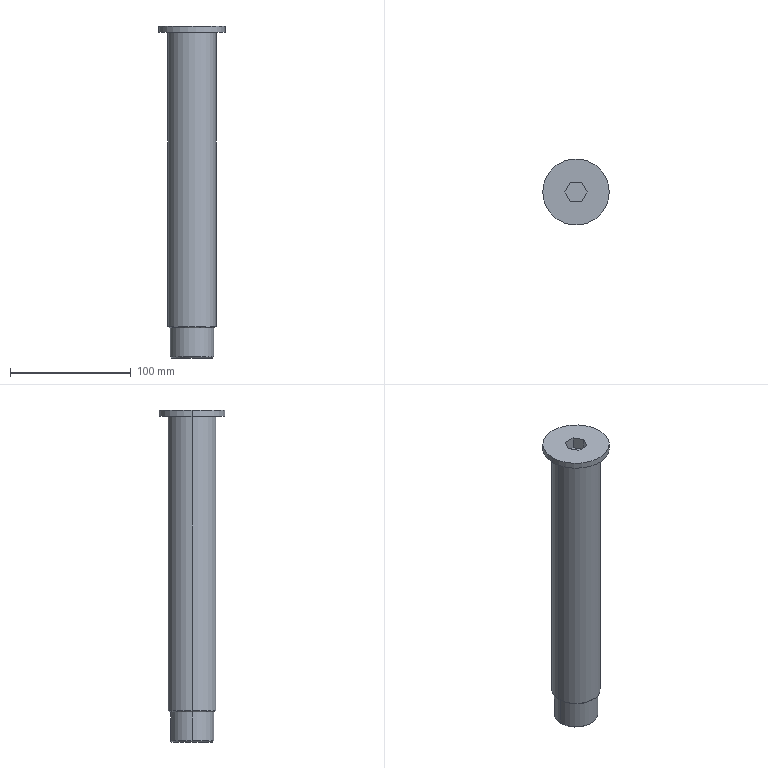Part | SolidWorks | features ICE 4, Chamfer 2, Fillet 2, Extrusion 1 | 1 solid | 32 faces | box 55 x 55 x 275 mm | volume 342139 mm3 | plane 14 | cylinder 11 | cone 5 | torus 2 | commonest cylinder face diameters 1 x4 36 x3 40 x2 55 x2
STEP:
#1=CARTESIAN_POINT('',(-20.5,0.,270.));
#2=VERTEX_POINT('',#1);
#3=CARTESIAN_POINT('',(20.5,0.,270.));
#4=VERTEX_POINT('',#3);
#5=CARTESIAN_POINT('',(0.,0.,270.));
#6=DIRECTION('',(0.,0.,1.));
#7=DIRECTION('',(1.,0.,0.));
#8=AXIS2_PLACEMENT_3D('',#5,#6,#7);
#9=CIRCLE('',#8,20.5);
#10=EDGE_CURVE('',#2,#4,#9,.T.);
#11=ORIENTED_EDGE('',*,*,#10,.F.);
#12=CARTESIAN_POINT('',(-20.,0.,269.5));
#13=VERTEX_POINT('',#12);
#14=CARTESIAN_POINT('',(-20.5,0.,269.5));
#15=DIRECTION('',(0.,1.,0.));
#16=DIRECTION('',(-1.,0.,0.));
#17=AXIS2_PLACEMENT_3D('',#14,#15,#16);
#18=CIRCLE('',#17,0.5);
#19=EDGE_CURVE('',#2,#13,#18,.T.);
#20=ORIENTED_EDGE('',*,*,#19,.T.);
#21=CARTESIAN_POINT('',(20.,0.,269.5));
#22=VERTEX_POINT('',#21);
#23=CARTESIAN_POINT('',(0.,0.,269.5));
#24=DIRECTION('',(0.,0.,-1.));
#25=DIRECTION('',(1.,0.,0.));
#26=AXIS2_PLACEMENT_3D('',#23,#24,#25);
#27=CIRCLE('',#26,20.);
#28=EDGE_CURVE('',#22,#13,#27,.T.);
#29=ORIENTED_EDGE('',*,*,#28,.F.);
#30=CARTESIAN_POINT('',(20.5,0.,269.5));
#31=DIRECTION('',(0.,-1.,0.));
#32=DIRECTION('',(0.,0.,-1.));
#33=AXIS2_PLACEMENT_3D('',#30,#31,#32);
#34=CIRCLE('',#33,0.5);
#35=EDGE_CURVE('',#4,#22,#34,.T.);
#36=ORIENTED_EDGE('',*,*,#35,.F.);
#37=EDGE_LOOP('',(#11,#20,#29,#36));
#38=FACE_OUTER_BOUND('',#37,.T.);
#39=CARTESIAN_POINT('',(0.,0.,269.5));
#40=DIRECTION('',(0.,0.,1.));
#41=DIRECTION('',(1.,0.,0.));
#42=AXIS2_PLACEMENT_3D('',#39,#40,#41);
#43=TOROIDAL_SURFACE('',#42,20.5,0.5);
#44=ADVANCED_FACE('',(#38),#43,.F.);
#45=CARTESIAN_POINT('',(-17.,0.,0.));
#46=VERTEX_POINT('',#45);
#47=CARTESIAN_POINT('',(-3.,16.733,0.));
#48=VERTEX_POINT('',#47);
#49=CARTESIAN_POINT('',(0.,0.,0.));
#50=DIRECTION('',(0.,0.,-1.));
#51=DIRECTION('',(1.,0.,0.));
#52=AXIS2_PLACEMENT_3D('',#49,#50,#51);
#53=CIRCLE('',#52,17.);
#54=EDGE_CURVE('',#46,#48,#53,.T.);
#55=ORIENTED_EDGE('',*,*,#54,.F.);
#56=CARTESIAN_POINT('',(-18.,0.,1.));
#57=VERTEX_POINT('',#56);
#58=CARTESIAN_POINT('',(-17.,0.,0.));
#59=DIRECTION('',(-0.7071,0.,0.7071));
#60=VECTOR('',#59,1000.);
#61=LINE('',#58,#60);
#62=EDGE_CURVE('',#46,#57,#61,.T.);
#63=ORIENTED_EDGE('',*,*,#62,.T.);
#64=CARTESIAN_POINT('',(-3.6,17.636,1.));
#65=VERTEX_POINT('',#64);
#66=CARTESIAN_POINT('',(0.,0.,1.));
#67=DIRECTION('',(0.,0.,1.));
#68=DIRECTION('',(1.,0.,0.));
#69=AXIS2_PLACEMENT_3D('',#66,#67,#68);
#70=CIRCLE('',#69,18.);
#71=EDGE_CURVE('',#65,#57,#70,.T.);
#72=ORIENTED_EDGE('',*,*,#71,.F.);
#73=CARTESIAN_POINT('',(-3.,17.146,0.4069));
#74=VERTEX_POINT('',#73);
#75=CARTESIAN_POINT('',(-3.6,17.636,1.));
#76=CARTESIAN_POINT('',(-3.509,17.655,1.));
#77=CARTESIAN_POINT('',(-3.418,17.647,0.9743));
#78=CARTESIAN_POINT('',(-3.262,17.594,0.8932));
#79=CARTESIAN_POINT('',(-3.198,17.551,0.8399));
#80=CARTESIAN_POINT('',(-3.098,17.452,0.7251));
#81=CARTESIAN_POINT('',(-3.061,17.395,0.6623));
#82=CARTESIAN_POINT('',(-3.013,17.275,0.5357));
#83=CARTESIAN_POINT('',(-3.,17.212,0.4712));
#84=CARTESIAN_POINT('',(-3.,17.146,0.4069));
#85=B_SPLINE_CURVE_WITH_KNOTS('',3,(#75,#76,#77,#78,#79,#80,#81,#82,#83,#84),.UNSPECIFIED.,.F.,.F.,(4,2,2,2,4),(0.,0.0002726,0.0005452,0.0008178,0.00109),.UNSPECIFIED.);
#86=EDGE_CURVE('',#65,#74,#85,.T.);
#87=ORIENTED_EDGE('',*,*,#86,.T.);
#88=CARTESIAN_POINT('',(-3.,16.733,0.));
#89=CARTESIAN_POINT('',(-3.,16.871,0.1356));
#90=CARTESIAN_POINT('',(-3.,17.009,0.2712));
#91=CARTESIAN_POINT('',(-3.,17.146,0.4069));
#92=B_SPLINE_CURVE_WITH_KNOTS('',3,(#88,#89,#90,#91),.UNSPECIFIED.,.F.,.F.,(4,4),(0.007295,0.007875),.UNSPECIFIED.);
#93=EDGE_CURVE('',#48,#74,#92,.T.);
#94=ORIENTED_EDGE('',*,*,#93,.F.);
#95=EDGE_LOOP('',(#55,#63,#72,#87,#94));
#96=FACE_OUTER_BOUND('',#95,.T.);
#97=CARTESIAN_POINT('',(0.,0.,0.));
#98=DIRECTION('',(0.,0.,1.));
#99=DIRECTION('',(1.,0.,0.));
#100=AXIS2_PLACEMENT_3D('',#97,#98,#99);
#101=CONICAL_SURFACE('',#100,17.,0.7854);
#102=ADVANCED_FACE('',(#96),#101,.T.);
#103=ORIENTED_EDGE('',*,*,#62,.F.);
#104=CARTESIAN_POINT('',(17.,0.,0.));
#105=VERTEX_POINT('',#104);
#106=CARTESIAN_POINT('',(0.,0.,0.));
#107=DIRECTION('',(0.,0.,-1.));
#108=DIRECTION('',(1.,0.,0.));
#109=AXIS2_PLACEMENT_3D('',#106,#107,#108);
#110=CIRCLE('',#109,17.);
#111=EDGE_CURVE('',#105,#46,#110,.T.);
#112=ORIENTED_EDGE('',*,*,#111,.F.);
#113=CARTESIAN_POINT('',(18.,0.,1.));
#114=VERTEX_POINT('',#113);
#115=CARTESIAN_POINT('',(17.,0.,0.));
#116=DIRECTION('',(0.7071,0.,0.7071));
#117=VECTOR('',#116,1000.);
#118=LINE('',#115,#117);
#119=EDGE_CURVE('',#105,#114,#118,.T.);
#120=ORIENTED_EDGE('',*,*,#119,.T.);
#121=CARTESIAN_POINT('',(0.,0.,1.));
#122=DIRECTION('',(0.,0.,1.));
#123=DIRECTION('',(1.,0.,0.));
#124=AXIS2_PLACEMENT_3D('',#121,#122,#123);
#125=CIRCLE('',#124,18.);
#126=EDGE_CURVE('',#57,#114,#125,.T.);
#127=ORIENTED_EDGE('',*,*,#126,.F.);
#128=EDGE_LOOP('',(#103,#112,#120,#127));
#129=FACE_OUTER_BOUND('',#128,.T.);
#130=CARTESIAN_POINT('',(0.,0.,0.));
#131=DIRECTION('',(0.,0.,1.));
#132=DIRECTION('',(1.,0.,0.));
#133=AXIS2_PLACEMENT_3D('',#130,#131,#132);
#134=CONICAL_SURFACE('',#133,17.,0.7854);
#135=ADVANCED_FACE('',(#129),#134,.T.);
#136=CARTESIAN_POINT('',(-19.,0.,25.));
#137=VERTEX_POINT('',#136);
#138=CARTESIAN_POINT('',(19.,0.,25.));
#139=VERTEX_POINT('',#138);
#140=CARTESIAN_POINT('',(0.,0.,25.));
#141=DIRECTION('',(0.,0.,-1.));
#142=DIRECTION('',(-1.,0.,0.));
#143=AXIS2_PLACEMENT_3D('',#140,#141,#142);
#144=CIRCLE('',#143,19.);
#145=EDGE_CURVE('',#137,#139,#144,.T.);
#146=ORIENTED_EDGE('',*,*,#145,.F.);
#147=CARTESIAN_POINT('',(-20.,0.,26.));
#148=VERTEX_POINT('',#147);
#149=CARTESIAN_POINT('',(-19.,0.,25.));
#150=DIRECTION('',(-0.7071,0.,0.7071));
#151=VECTOR('',#150,1000.);
#152=LINE('',#149,#151);
#153=EDGE_CURVE('',#137,#148,#152,.T.);
#154=ORIENTED_EDGE('',*,*,#153,.T.);
#155=CARTESIAN_POINT('',(20.,0.,26.));
#156=VERTEX_POINT('',#155);
#157=CARTESIAN_POINT('',(0.,0.,26.));
#158=DIRECTION('',(0.,0.,1.));
#159=DIRECTION('',(-1.,0.,0.));
#160=AXIS2_PLACEMENT_3D('',#157,#158,#159);
#161=CIRCLE('',#160,20.);
#162=EDGE_CURVE('',#156,#148,#161,.T.);
#163=ORIENTED_EDGE('',*,*,#162,.F.);
#164=CARTESIAN_POINT('',(19.,0.,25.));
#165=DIRECTION('',(0.7071,0.,0.7071));
#166=VECTOR('',#165,1000.);
#167=LINE('',#164,#166);
#168=EDGE_CURVE('',#139,#156,#167,.T.);
#169=ORIENTED_EDGE('',*,*,#168,.F.);
#170=EDGE_LOOP('',(#146,#154,#163,#169));
#171=FACE_OUTER_BOUND('',#170,.T.);
#172=CARTESIAN_POINT('',(0.,0.,25.));
#173=DIRECTION('',(0.,0.,1.));
#174=DIRECTION('',(1.,0.,0.));
#175=AXIS2_PLACEMENT_3D('',#172,#173,#174);
#176=CONICAL_SURFACE('',#175,19.,0.7854);
#177=ADVANCED_FACE('',(#171),#176,.T.);
#178=CARTESIAN_POINT('',(3.6,17.636,25.));
#179=VERTEX_POINT('',#178);
#180=CARTESIAN_POINT('',(18.,0.,25.));
#181=VERTEX_POINT('',#180);
#182=CARTESIAN_POINT('',(0.,0.,25.));
#183=DIRECTION('',(0.,0.,-1.));
#184=DIRECTION('',(-1.,0.,0.));
#185=AXIS2_PLACEMENT_3D('',#182,#183,#184);
#186=CIRCLE('',#185,18.);
#187=EDGE_CURVE('',#179,#181,#186,.T.);
#188=ORIENTED_EDGE('',*,*,#187,.T.);
#189=CARTESIAN_POINT('',(18.,0.,25.));
#190=DIRECTION('',(0.,0.,-1.));
#191=VECTOR('',#190,1000.);
#192=LINE('',#189,#191);
#193=EDGE_CURVE('',#181,#114,#192,.T.);
#194=ORIENTED_EDGE('',*,*,#193,.T.);
#195=CARTESIAN_POINT('',(3.6,17.636,1.));
#196=VERTEX_POINT('',#195);
#197=CARTESIAN_POINT('',(0.,0.,1.));
#198=DIRECTION('',(0.,0.,1.));
#199=DIRECTION('',(1.,0.,0.));
#200=AXIS2_PLACEMENT_3D('',#197,#198,#199);
#201=CIRCLE('',#200,18.);
#202=EDGE_CURVE('',#114,#196,#201,.T.);
#203=ORIENTED_EDGE('',*,*,#202,.T.);
#204=CARTESIAN_POINT('',(3.6,17.636,25.));
#205=DIRECTION('',(0.,0.,1.));
#206=VECTOR('',#205,1000.);
#207=LINE('',#204,#206);
#208=EDGE_CURVE('',#196,#179,#207,.T.);
#209=ORIENTED_EDGE('',*,*,#208,.T.);
#210=EDGE_LOOP('',(#188,#194,#203,#209));
#211=FACE_OUTER_BOUND('',#210,.T.);
#212=CARTESIAN_POINT('',(0.,0.,25.));
#213=DIRECTION('',(0.,0.,-1.));
#214=DIRECTION('',(-1.,0.,0.));
#215=AXIS2_PLACEMENT_3D('',#212,#213,#214);
#216=CYLINDRICAL_SURFACE('',#215,18.);
#217=ADVANCED_FACE('',(#211),#216,.T.);
#218=ORIENTED_EDGE('',*,*,#193,.F.);
#219=CARTESIAN_POINT('',(-18.,0.,25.));
#220=VERTEX_POINT('',#219);
#221=CARTESIAN_POINT('',(0.,0.,25.));
#222=DIRECTION('',(0.,0.,-1.));
#223=DIRECTION('',(-1.,0.,0.));
#224=AXIS2_PLACEMENT_3D('',#221,#222,#223);
#225=CIRCLE('',#224,18.);
#226=EDGE_CURVE('',#181,#220,#225,.T.);
#227=ORIENTED_EDGE('',*,*,#226,.T.);
#228=CARTESIAN_POINT('',(-18.,0.,25.));
#229=DIRECTION('',(0.,0.,-1.));
#230=VECTOR('',#229,1000.);
#231=LINE('',#228,#230);
#232=EDGE_CURVE('',#220,#57,#231,.T.);
#233=ORIENTED_EDGE('',*,*,#232,.T.);
#234=ORIENTED_EDGE('',*,*,#126,.T.);
#235=EDGE_LOOP('',(#218,#227,#233,#234));
#236=FACE_OUTER_BOUND('',#235,.T.);
#237=CARTESIAN_POINT('',(0.,0.,25.));
#238=DIRECTION('',(0.,0.,-1.));
#239=DIRECTION('',(-1.,0.,0.));
#240=AXIS2_PLACEMENT_3D('',#237,#238,#239);
#241=CYLINDRICAL_SURFACE('',#240,18.);
#242=ADVANCED_FACE('',(#236),#241,.T.);
#243=CARTESIAN_POINT('',(27.5,0.,275.));
#244=VERTEX_POINT('',#243);
#245=CARTESIAN_POINT('',(-27.5,0.,275.));
#246=VERTEX_POINT('',#245);
#247=CARTESIAN_POINT('',(0.,0.,275.));
#248=DIRECTION('',(0.,0.,1.));
#249=DIRECTION('',(1.,0.,0.));
#250=AXIS2_PLACEMENT_3D('',#247,#248,#249);
#251=CIRCLE('',#250,27.5);
#252=EDGE_CURVE('',#244,#246,#251,.T.);
#253=ORIENTED_EDGE('',*,*,#252,.F.);
#254=CARTESIAN_POINT('',(27.5,0.,270.));
#255=VERTEX_POINT('',#254);
#256=CARTESIAN_POINT('',(27.5,0.,275.));
#257=DIRECTION('',(0.,0.,-1.));
#258=VECTOR('',#257,1000.);
#259=LINE('',#256,#258);
#260=EDGE_CURVE('',#244,#255,#259,.T.);
#261=ORIENTED_EDGE('',*,*,#260,.T.);
#262=CARTESIAN_POINT('',(-27.5,0.,270.));
#263=VERTEX_POINT('',#262);
#264=CARTESIAN_POINT('',(0.,0.,270.));
#265=DIRECTION('',(0.,0.,1.));
#266=DIRECTION('',(1.,0.,0.));
#267=AXIS2_PLACEMENT_3D('',#264,#265,#266);
#268=CIRCLE('',#267,27.5);
#269=EDGE_CURVE('',#255,#263,#268,.T.);
#270=ORIENTED_EDGE('',*,*,#269,.T.);
#271=CARTESIAN_POINT('',(-27.5,0.,275.));
#272=DIRECTION('',(0.,0.,-1.));
#273=VECTOR('',#272,1000.);
#274=LINE('',#271,#273);
#275=EDGE_CURVE('',#246,#263,#274,.T.);
#276=ORIENTED_EDGE('',*,*,#275,.F.);
#277=EDGE_LOOP('',(#253,#261,#270,#276));
#278=FACE_OUTER_BOUND('',#277,.T.);
#279=CARTESIAN_POINT('',(0.,0.,275.));
#280=DIRECTION('',(0.,0.,-1.));
#281=DIRECTION('',(-1.,0.,0.));
#282=AXIS2_PLACEMENT_3D('',#279,#280,#281);
#283=CYLINDRICAL_SURFACE('',#282,27.5);
#284=ADVANCED_FACE('',(#278),#283,.T.);
#285=CARTESIAN_POINT('',(0.,0.,269.5));
#286=DIRECTION('',(0.,0.,-1.));
#287=DIRECTION('',(1.,0.,0.));
#288=AXIS2_PLACEMENT_3D('',#285,#286,#287);
#289=CIRCLE('',#288,20.);
#290=EDGE_CURVE('',#13,#22,#289,.T.);
#291=ORIENTED_EDGE('',*,*,#290,.T.);
#292=CARTESIAN_POINT('',(20.,0.,270.));
#293=DIRECTION('',(0.,0.,-1.));
#294=VECTOR('',#293,1000.);
#295=LINE('',#292,#294);
#296=EDGE_CURVE('',#22,#156,#295,.T.);
#297=ORIENTED_EDGE('',*,*,#296,.T.);
#298=ORIENTED_EDGE('',*,*,#162,.T.);
#299=CARTESIAN_POINT('',(-20.,0.,270.));
#300=DIRECTION('',(0.,0.,-1.));
#301=VECTOR('',#300,1000.);
#302=LINE('',#299,#301);
#303=EDGE_CURVE('',#13,#148,#302,.T.);
#304=ORIENTED_EDGE('',*,*,#303,.F.);
#305=EDGE_LOOP('',(#291,#297,#298,#304));
#306=FACE_OUTER_BOUND('',#305,.T.);
#307=CARTESIAN_POINT('',(0.,0.,270.));
#308=DIRECTION('',(0.,0.,-1.));
#309=DIRECTION('',(-1.,0.,0.));
#310=AXIS2_PLACEMENT_3D('',#307,#308,#309);
#311=CYLINDRICAL_SURFACE('',#310,20.);
#312=ADVANCED_FACE('',(#306),#311,.T.);
#313=ORIENTED_EDGE('',*,*,#296,.F.);
#314=ORIENTED_EDGE('',*,*,#28,.T.);
#315=ORIENTED_EDGE('',*,*,#303,.T.);
#316=CARTESIAN_POINT('',(0.,0.,26.));
#317=DIRECTION('',(0.,0.,1.));
#318=DIRECTION('',(-1.,0.,0.));
#319=AXIS2_PLACEMENT_3D('',#316,#317,#318);
#320=CIRCLE('',#319,20.);
#321=EDGE_CURVE('',#148,#156,#320,.T.);
#322=ORIENTED_EDGE('',*,*,#321,.T.);
#323=EDGE_LOOP('',(#313,#314,#315,#322));
#324=FACE_OUTER_BOUND('',#323,.T.);
#325=CARTESIAN_POINT('',(0.,0.,270.));
#326=DIRECTION('',(0.,0.,-1.));
#327=DIRECTION('',(-1.,0.,0.));
#328=AXIS2_PLACEMENT_3D('',#325,#326,#327);
#329=CYLINDRICAL_SURFACE('',#328,20.);
#330=ADVANCED_FACE('',(#324),#329,.T.);
#331=ORIENTED_EDGE('',*,*,#260,.F.);
#332=CARTESIAN_POINT('',(0.,0.,275.));
#333=DIRECTION('',(0.,0.,1.));
#334=DIRECTION('',(1.,0.,0.));
#335=AXIS2_PLACEMENT_3D('',#332,#333,#334);
#336=CIRCLE('',#335,27.5);
#337=EDGE_CURVE('',#246,#244,#336,.T.);
#338=ORIENTED_EDGE('',*,*,#337,.F.);
#339=ORIENTED_EDGE('',*,*,#275,.T.);
#340=CARTESIAN_POINT('',(0.,0.,270.));
#341=DIRECTION('',(0.,0.,1.));
#342=DIRECTION('',(1.,0.,0.));
#343=AXIS2_PLACEMENT_3D('',#340,#341,#342);
#344=CIRCLE('',#343,27.5);
#345=EDGE_CURVE('',#263,#255,#344,.T.);
#346=ORIENTED_EDGE('',*,*,#345,.T.);
#347=EDGE_LOOP('',(#331,#338,#339,#346));
#348=FACE_OUTER_BOUND('',#347,.T.);
#349=CARTESIAN_POINT('',(0.,0.,275.));
#350=DIRECTION('',(0.,0.,-1.));
#351=DIRECTION('',(-1.,0.,0.));
#352=AXIS2_PLACEMENT_3D('',#349,#350,#351);
#353=CYLINDRICAL_SURFACE('',#352,27.5);
#354=ADVANCED_FACE('',(#348),#353,.T.);
#355=CARTESIAN_POINT('',(4.619,-8.,275.));
#356=VERTEX_POINT('',#355);
#357=CARTESIAN_POINT('',(9.238,0.,275.));
#358=VERTEX_POINT('',#357);
#359=CARTESIAN_POINT('',(4.619,-8.,275.));
#360=DIRECTION('',(0.5,0.866,0.));
#361=VECTOR('',#360,1000.);
#362=LINE('',#359,#361);
#363=EDGE_CURVE('',#356,#358,#362,.T.);
#364=ORIENTED_EDGE('',*,*,#363,.F.);
#365=CARTESIAN_POINT('',(-4.619,-8.,275.));
#366=VERTEX_POINT('',#365);
#367=CARTESIAN_POINT('',(-4.619,-8.,275.));
#368=DIRECTION('',(1.,0.,0.));
#369=VECTOR('',#368,1000.);
#370=LINE('',#367,#369);
#371=EDGE_CURVE('',#366,#356,#370,.T.);
#372=ORIENTED_EDGE('',*,*,#371,.F.);
#373=CARTESIAN_POINT('',(-9.238,0.,275.));
#374=VERTEX_POINT('',#373);
#375=CARTESIAN_POINT('',(-9.238,0.,275.));
#376=DIRECTION('',(0.5,-0.866,0.));
#377=VECTOR('',#376,1000.);
#378=LINE('',#375,#377);
#379=EDGE_CURVE('',#374,#366,#378,.T.);
#380=ORIENTED_EDGE('',*,*,#379,.F.);
#381=CARTESIAN_POINT('',(-4.619,8.,275.));
#382=VERTEX_POINT('',#381);
#383=CARTESIAN_POINT('',(-4.619,8.,275.));
#384=DIRECTION('',(-0.5,-0.866,0.));
#385=VECTOR('',#384,1000.);
#386=LINE('',#383,#385);
#387=EDGE_CURVE('',#382,#374,#386,.T.);
#388=ORIENTED_EDGE('',*,*,#387,.F.);
#389=CARTESIAN_POINT('',(4.619,8.,275.));
#390=VERTEX_POINT('',#389);
#391=CARTESIAN_POINT('',(4.619,8.,275.));
#392=DIRECTION('',(-1.,0.,0.));
#393=VECTOR('',#392,1000.);
#394=LINE('',#391,#393);
#395=EDGE_CURVE('',#390,#382,#394,.T.);
#396=ORIENTED_EDGE('',*,*,#395,.F.);
#397=CARTESIAN_POINT('',(9.238,0.,275.));
#398=DIRECTION('',(-0.5,0.866,0.));
#399=VECTOR('',#398,1000.);
#400=LINE('',#397,#399);
#401=EDGE_CURVE('',#358,#390,#400,.T.);
#402=ORIENTED_EDGE('',*,*,#401,.F.);
#403=EDGE_LOOP('',(#364,#372,#380,#388,#396,#402));
#404=FACE_BOUND('',#403,.T.);
#405=ORIENTED_EDGE('',*,*,#337,.T.);
#406=ORIENTED_EDGE('',*,*,#252,.T.);
#407=EDGE_LOOP('',(#405,#406));
#408=FACE_OUTER_BOUND('',#407,.T.);
#409=CARTESIAN_POINT('',(0.,0.,275.));
#410=DIRECTION('',(0.,0.,1.));
#411=DIRECTION('',(1.,0.,0.));
#412=AXIS2_PLACEMENT_3D('',#409,#410,#411);
#413=PLANE('',#412);
#414=ADVANCED_FACE('',(#404,#408),#413,.T.);
#415=CARTESIAN_POINT('',(0.,0.,270.));
#416=DIRECTION('',(0.,0.,1.));
#417=DIRECTION('',(1.,0.,0.));
#418=AXIS2_PLACEMENT_3D('',#415,#416,#417);
#419=CIRCLE('',#418,20.5);
#420=EDGE_CURVE('',#4,#2,#419,.T.);
#421=ORIENTED_EDGE('',*,*,#420,.T.);
#422=ORIENTED_EDGE('',*,*,#10,.T.);
#423=EDGE_LOOP('',(#421,#422));
#424=FACE_BOUND('',#423,.T.);
#425=ORIENTED_EDGE('',*,*,#345,.F.);
#426=ORIENTED_EDGE('',*,*,#269,.F.);
#427=EDGE_LOOP('',(#425,#426));
#428=FACE_OUTER_BOUND('',#427,.T.);
#429=CARTESIAN_POINT('',(0.,0.,270.));
#430=DIRECTION('',(0.,0.,1.));
#431=DIRECTION('',(1.,0.,0.));
#432=AXIS2_PLACEMENT_3D('',#429,#430,#431);
#433=PLANE('',#432);
#434=ADVANCED_FACE('',(#424,#428),#433,.F.);
#435=ORIENTED_EDGE('',*,*,#363,.T.);
#436=CARTESIAN_POINT('',(9.238,0.,265.));
#437=VERTEX_POINT('',#436);
#438=CARTESIAN_POINT('',(9.238,0.,265.));
#439=DIRECTION('',(0.,0.,1.));
#440=VECTOR('',#439,1000.);
#441=LINE('',#438,#440);
#442=EDGE_CURVE('',#437,#358,#441,.T.);
#443=ORIENTED_EDGE('',*,*,#442,.F.);
#444=CARTESIAN_POINT('',(4.619,-8.,265.));
#445=VERTEX_POINT('',#444);
#446=CARTESIAN_POINT('',(4.619,-8.,265.));
#447=DIRECTION('',(0.5,0.866,0.));
#448=VECTOR('',#447,1000.);
#449=LINE('',#446,#448);
#450=EDGE_CURVE('',#445,#437,#449,.T.);
#451=ORIENTED_EDGE('',*,*,#450,.F.);
#452=CARTESIAN_POINT('',(4.619,-8.,265.));
#453=DIRECTION('',(0.,0.,1.));
#454=VECTOR('',#453,1000.);
#455=LINE('',#452,#454);
#456=EDGE_CURVE('',#445,#356,#455,.T.);
#457=ORIENTED_EDGE('',*,*,#456,.T.);
#458=EDGE_LOOP('',(#435,#443,#451,#457));
#459=FACE_OUTER_BOUND('',#458,.T.);
#460=CARTESIAN_POINT('',(4.619,-8.,265.));
#461=DIRECTION('',(0.866,-0.5,0.));
#462=DIRECTION('',(0.5,0.866,0.));
#463=AXIS2_PLACEMENT_3D('',#460,#461,#462);
#464=PLANE('',#463);
#465=ADVANCED_FACE('',(#459),#464,.F.);
#466=ORIENTED_EDGE('',*,*,#371,.T.);
#467=ORIENTED_EDGE('',*,*,#456,.F.);
#468=CARTESIAN_POINT('',(-4.619,-8.,265.));
#469=VERTEX_POINT('',#468);
#470=CARTESIAN_POINT('',(-4.619,-8.,265.));
#471=DIRECTION('',(1.,0.,0.));
#472=VECTOR('',#471,1000.);
#473=LINE('',#470,#472);
#474=EDGE_CURVE('',#469,#445,#473,.T.);
#475=ORIENTED_EDGE('',*,*,#474,.F.);
#476=CARTESIAN_POINT('',(-4.619,-8.,265.));
#477=DIRECTION('',(0.,0.,1.));
#478=VECTOR('',#477,1000.);
#479=LINE('',#476,#478);
#480=EDGE_CURVE('',#469,#366,#479,.T.);
#481=ORIENTED_EDGE('',*,*,#480,.T.);
#482=EDGE_LOOP('',(#466,#467,#475,#481));
#483=FACE_OUTER_BOUND('',#482,.T.);
#484=CARTESIAN_POINT('',(-4.619,-8.,265.));
#485=DIRECTION('',(0.,-1.,0.));
#486=DIRECTION('',(1.,0.,0.));
#487=AXIS2_PLACEMENT_3D('',#484,#485,#486);
#488=PLANE('',#487);
#489=ADVANCED_FACE('',(#483),#488,.F.);
#490=ORIENTED_EDGE('',*,*,#379,.T.);
#491=ORIENTED_EDGE('',*,*,#480,.F.);
#492=CARTESIAN_POINT('',(-9.238,0.,265.));
#493=VERTEX_POINT('',#492);
#494=CARTESIAN_POINT('',(-9.238,0.,265.));
#495=DIRECTION('',(0.5,-0.866,0.));
#496=VECTOR('',#495,1000.);
#497=LINE('',#494,#496);
#498=EDGE_CURVE('',#493,#469,#497,.T.);
#499=ORIENTED_EDGE('',*,*,#498,.F.);
#500=CARTESIAN_POINT('',(-9.238,0.,265.));
#501=DIRECTION('',(0.,0.,1.));
#502=VECTOR('',#501,1000.);
#503=LINE('',#500,#502);
#504=EDGE_CURVE('',#493,#374,#503,.T.);
#505=ORIENTED_EDGE('',*,*,#504,.T.);
#506=EDGE_LOOP('',(#490,#491,#499,#505));
#507=FACE_OUTER_BOUND('',#506,.T.);
#508=CARTESIAN_POINT('',(-9.238,0.,265.));
#509=DIRECTION('',(-0.866,-0.5,0.));
#510=DIRECTION('',(0.5,-0.866,0.));
#511=AXIS2_PLACEMENT_3D('',#508,#509,#510);
#512=PLANE('',#511);
#513=ADVANCED_FACE('',(#507),#512,.F.);
#514=ORIENTED_EDGE('',*,*,#387,.T.);
#515=ORIENTED_EDGE('',*,*,#504,.F.);
#516=CARTESIAN_POINT('',(-4.619,8.,265.));
#517=VERTEX_POINT('',#516);
#518=CARTESIAN_POINT('',(-4.619,8.,265.));
#519=DIRECTION('',(-0.5,-0.866,0.));
#520=VECTOR('',#519,1000.);
#521=LINE('',#518,#520);
#522=EDGE_CURVE('',#517,#493,#521,.T.);
#523=ORIENTED_EDGE('',*,*,#522,.F.);
#524=CARTESIAN_POINT('',(-4.619,8.,265.));
#525=DIRECTION('',(0.,0.,1.));
#526=VECTOR('',#525,1000.);
#527=LINE('',#524,#526);
#528=EDGE_CURVE('',#517,#382,#527,.T.);
#529=ORIENTED_EDGE('',*,*,#528,.T.);
#530=EDGE_LOOP('',(#514,#515,#523,#529));
#531=FACE_OUTER_BOUND('',#530,.T.);
#532=CARTESIAN_POINT('',(-4.619,8.,265.));
#533=DIRECTION('',(-0.866,0.5,0.));
#534=DIRECTION('',(-0.5,-0.866,0.));
#535=AXIS2_PLACEMENT_3D('',#532,#533,#534);
#536=PLANE('',#535);
#537=ADVANCED_FACE('',(#531),#536,.F.);
#538=ORIENTED_EDGE('',*,*,#395,.T.);
#539=ORIENTED_EDGE('',*,*,#528,.F.);
#540=CARTESIAN_POINT('',(4.619,8.,265.));
#541=VERTEX_POINT('',#540);
#542=CARTESIAN_POINT('',(4.619,8.,265.));
#543=DIRECTION('',(-1.,0.,0.));
#544=VECTOR('',#543,1000.);
#545=LINE('',#542,#544);
#546=EDGE_CURVE('',#541,#517,#545,.T.);
#547=ORIENTED_EDGE('',*,*,#546,.F.);
#548=CARTESIAN_POINT('',(4.619,8.,265.));
#549=DIRECTION('',(0.,0.,1.));
#550=VECTOR('',#549,1000.);
#551=LINE('',#548,#550);
#552=EDGE_CURVE('',#541,#390,#551,.T.);
#553=ORIENTED_EDGE('',*,*,#552,.T.);
#554=EDGE_LOOP('',(#538,#539,#547,#553));
#555=FACE_OUTER_BOUND('',#554,.T.);
#556=CARTESIAN_POINT('',(4.619,8.,265.));
#557=DIRECTION('',(0.,1.,0.));
#558=DIRECTION('',(0.,0.,1.));
#559=AXIS2_PLACEMENT_3D('',#556,#557,#558);
#560=PLANE('',#559);
#561=ADVANCED_FACE('',(#555),#560,.F.);
#562=ORIENTED_EDGE('',*,*,#401,.T.);
#563=ORIENTED_EDGE('',*,*,#552,.F.);
#564=CARTESIAN_POINT('',(9.238,0.,265.));
#565=DIRECTION('',(-0.5,0.866,0.));
#566=VECTOR('',#565,1000.);
#567=LINE('',#564,#566);
#568=EDGE_CURVE('',#437,#541,#567,.T.);
#569=ORIENTED_EDGE('',*,*,#568,.F.);
#570=ORIENTED_EDGE('',*,*,#442,.T.);
#571=EDGE_LOOP('',(#562,#563,#569,#570));
#572=FACE_OUTER_BOUND('',#571,.T.);
#573=CARTESIAN_POINT('',(9.238,0.,265.));
#574=DIRECTION('',(0.866,0.5,0.));
#575=DIRECTION('',(-0.5,0.866,0.));
#576=AXIS2_PLACEMENT_3D('',#573,#574,#575);
#577=PLANE('',#576);
#578=ADVANCED_FACE('',(#572),#577,.F.);
#579=ORIENTED_EDGE('',*,*,#450,.T.);
#580=ORIENTED_EDGE('',*,*,#568,.T.);
#581=ORIENTED_EDGE('',*,*,#546,.T.);
#582=ORIENTED_EDGE('',*,*,#522,.T.);
#583=ORIENTED_EDGE('',*,*,#498,.T.);
#584=ORIENTED_EDGE('',*,*,#474,.T.);
#585=EDGE_LOOP('',(#579,#580,#581,#582,#583,#584));
#586=FACE_OUTER_BOUND('',#585,.T.);
#587=CARTESIAN_POINT('',(0.,0.,265.));
#588=DIRECTION('',(0.,0.,1.));
#589=DIRECTION('',(1.,0.,0.));
#590=AXIS2_PLACEMENT_3D('',#587,#588,#589);
#591=PLANE('',#590);
#592=ADVANCED_FACE('',(#586),#591,.T.);
#593=CARTESIAN_POINT('',(0.,0.,25.));
#594=DIRECTION('',(0.,0.,-1.));
#595=DIRECTION('',(-1.,0.,0.));
#596=AXIS2_PLACEMENT_3D('',#593,#594,#595);
#597=CIRCLE('',#596,19.);
#598=EDGE_CURVE('',#139,#137,#597,.T.);
#599=ORIENTED_EDGE('',*,*,#598,.T.);
#600=ORIENTED_EDGE('',*,*,#145,.T.);
#601=EDGE_LOOP('',(#599,#600));
#602=FACE_OUTER_BOUND('',#601,.T.);
#603=CARTESIAN_POINT('',(3.,13.5,25.));
#604=VERTEX_POINT('',#603);
#605=CARTESIAN_POINT('',(3.,17.146,25.));
#606=VERTEX_POINT('',#605);
#607=CARTESIAN_POINT('',(3.,23.,25.));
#608=DIRECTION('',(0.,1.,0.));
#609=VECTOR('',#608,1000.);
#610=LINE('',#607,#609);
#611=EDGE_CURVE('',#604,#606,#610,.T.);
#612=ORIENTED_EDGE('',*,*,#611,.F.);
#613=CARTESIAN_POINT('',(2.5,13.,25.));
#614=VERTEX_POINT('',#613);
#615=CARTESIAN_POINT('',(2.5,13.5,25.));
#616=DIRECTION('',(0.,0.,-1.));
#617=DIRECTION('',(-1.,0.,0.));
#618=AXIS2_PLACEMENT_3D('',#615,#616,#617);
#619=CIRCLE('',#618,0.5);
#620=EDGE_CURVE('',#604,#614,#619,.T.);
#621=ORIENTED_EDGE('',*,*,#620,.T.);
#622=CARTESIAN_POINT('',(-2.5,13.,25.));
#623=VERTEX_POINT('',#622);
#624=CARTESIAN_POINT('',(3.,13.,25.));
#625=DIRECTION('',(1.,0.,0.));
#626=VECTOR('',#625,1000.);
#627=LINE('',#624,#626);
#628=EDGE_CURVE('',#623,#614,#627,.T.);
#629=ORIENTED_EDGE('',*,*,#628,.F.);
#630=CARTESIAN_POINT('',(-3.,13.5,25.));
#631=VERTEX_POINT('',#630);
#632=CARTESIAN_POINT('',(-2.5,13.5,25.));
#633=DIRECTION('',(0.,0.,-1.));
#634=DIRECTION('',(-1.,0.,0.));
#635=AXIS2_PLACEMENT_3D('',#632,#633,#634);
#636=CIRCLE('',#635,0.5);
#637=EDGE_CURVE('',#623,#631,#636,.T.);
#638=ORIENTED_EDGE('',*,*,#637,.T.);
#639=CARTESIAN_POINT('',(-3.,17.146,25.));
#640=VERTEX_POINT('',#639);
#641=CARTESIAN_POINT('',(-3.,23.,25.));
#642=DIRECTION('',(0.,-1.,0.));
#643=VECTOR('',#642,1000.);
#644=LINE('',#641,#643);
#645=EDGE_CURVE('',#640,#631,#644,.T.);
#646=ORIENTED_EDGE('',*,*,#645,.F.);
#647=CARTESIAN_POINT('',(-3.6,17.636,25.));
#648=VERTEX_POINT('',#647);
#649=CARTESIAN_POINT('',(-3.5,17.146,25.));
#650=DIRECTION('',(0.,0.,1.));
#651=DIRECTION('',(-1.,0.,0.));
#652=AXIS2_PLACEMENT_3D('',#649,#650,#651);
#653=CIRCLE('',#652,0.5);
#654=EDGE_CURVE('',#640,#648,#653,.T.);
#655=ORIENTED_EDGE('',*,*,#654,.T.);
#656=CARTESIAN_POINT('',(0.,0.,25.));
#657=DIRECTION('',(0.,0.,-1.));
#658=DIRECTION('',(-1.,0.,0.));
#659=AXIS2_PLACEMENT_3D('',#656,#657,#658);
#660=CIRCLE('',#659,18.);
#661=EDGE_CURVE('',#220,#648,#660,.T.);
#662=ORIENTED_EDGE('',*,*,#661,.F.);
#663=ORIENTED_EDGE('',*,*,#226,.F.);
#664=ORIENTED_EDGE('',*,*,#187,.F.);
#665=CARTESIAN_POINT('',(3.5,17.146,25.));
#666=DIRECTION('',(0.,0.,1.));
#667=DIRECTION('',(-1.,0.,0.));
#668=AXIS2_PLACEMENT_3D('',#665,#666,#667);
#669=CIRCLE('',#668,0.5);
#670=EDGE_CURVE('',#179,#606,#669,.T.);
#671=ORIENTED_EDGE('',*,*,#670,.T.);
#672=EDGE_LOOP('',(#612,#621,#629,#638,#646,#655,#662,#663,#664,#671));
#673=FACE_BOUND('',#672,.T.);
#674=CARTESIAN_POINT('',(0.,0.,25.));
#675=DIRECTION('',(0.,0.,-1.));
#676=DIRECTION('',(-1.,0.,0.));
#677=AXIS2_PLACEMENT_3D('',#674,#675,#676);
#678=PLANE('',#677);
#679=ADVANCED_FACE('',(#602,#673),#678,.T.);
#680=ORIENTED_EDGE('',*,*,#232,.F.);
#681=ORIENTED_EDGE('',*,*,#661,.T.);
#682=CARTESIAN_POINT('',(-3.6,17.636,25.));
#683=DIRECTION('',(0.,0.,-1.));
#684=VECTOR('',#683,1000.);
#685=LINE('',#682,#684);
#686=EDGE_CURVE('',#648,#65,#685,.T.);
#687=ORIENTED_EDGE('',*,*,#686,.T.);
#688=ORIENTED_EDGE('',*,*,#71,.T.);
#689=EDGE_LOOP('',(#680,#681,#687,#688));
#690=FACE_OUTER_BOUND('',#689,.T.);
#691=CARTESIAN_POINT('',(0.,0.,25.));
#692=DIRECTION('',(0.,0.,-1.));
#693=DIRECTION('',(-1.,0.,0.));
#694=AXIS2_PLACEMENT_3D('',#691,#692,#693);
#695=CYLINDRICAL_SURFACE('',#694,18.);
#696=ADVANCED_FACE('',(#690),#695,.T.);
#697=CARTESIAN_POINT('',(3.,16.733,0.));
#698=VERTEX_POINT('',#697);
#699=CARTESIAN_POINT('',(0.,0.,0.));
#700=DIRECTION('',(0.,0.,-1.));
#701=DIRECTION('',(1.,0.,0.));
#702=AXIS2_PLACEMENT_3D('',#699,#700,#701);
#703=CIRCLE('',#702,17.);
#704=EDGE_CURVE('',#698,#105,#703,.T.);
#705=ORIENTED_EDGE('',*,*,#704,.T.);
#706=ORIENTED_EDGE('',*,*,#111,.T.);
#707=ORIENTED_EDGE('',*,*,#54,.T.);
#708=CARTESIAN_POINT('',(-3.,13.5,0.));
#709=VERTEX_POINT('',#708);
#710=CARTESIAN_POINT('',(-3.,23.,0.));
#711=DIRECTION('',(0.,1.,0.));
#712=VECTOR('',#711,1000.);
#713=LINE('',#710,#712);
#714=EDGE_CURVE('',#709,#48,#713,.T.);
#715=ORIENTED_EDGE('',*,*,#714,.F.);
#716=CARTESIAN_POINT('',(-2.5,13.,0.));
#717=VERTEX_POINT('',#716);
#718=CARTESIAN_POINT('',(-2.5,13.5,0.));
#719=DIRECTION('',(0.,0.,1.));
#720=DIRECTION('',(1.,0.,0.));
#721=AXIS2_PLACEMENT_3D('',#718,#719,#720);
#722=CIRCLE('',#721,0.5);
#723=EDGE_CURVE('',#709,#717,#722,.T.);
#724=ORIENTED_EDGE('',*,*,#723,.T.);
#725=CARTESIAN_POINT('',(2.5,13.,0.));
#726=VERTEX_POINT('',#725);
#727=CARTESIAN_POINT('',(3.,13.,0.));
#728=DIRECTION('',(-1.,0.,0.));
#729=VECTOR('',#728,1000.);
#730=LINE('',#727,#729);
#731=EDGE_CURVE('',#726,#717,#730,.T.);
#732=ORIENTED_EDGE('',*,*,#731,.F.);
#733=CARTESIAN_POINT('',(3.,13.5,0.));
#734=VERTEX_POINT('',#733);
#735=CARTESIAN_POINT('',(2.5,13.5,0.));
#736=DIRECTION('',(0.,0.,1.));
#737=DIRECTION('',(1.,0.,0.));
#738=AXIS2_PLACEMENT_3D('',#735,#736,#737);
#739=CIRCLE('',#738,0.5);
#740=EDGE_CURVE('',#726,#734,#739,.T.);
#741=ORIENTED_EDGE('',*,*,#740,.T.);
#742=CARTESIAN_POINT('',(3.,23.,0.));
#743=DIRECTION('',(0.,-1.,0.));
#744=VECTOR('',#743,1000.);
#745=LINE('',#742,#744);
#746=EDGE_CURVE('',#698,#734,#745,.T.);
#747=ORIENTED_EDGE('',*,*,#746,.F.);
#748=EDGE_LOOP('',(#705,#706,#707,#715,#724,#732,#741,#747));
#749=FACE_OUTER_BOUND('',#748,.T.);
#750=CARTESIAN_POINT('',(0.,0.,0.));
#751=DIRECTION('',(0.,0.,1.));
#752=DIRECTION('',(1.,0.,0.));
#753=AXIS2_PLACEMENT_3D('',#750,#751,#752);
#754=PLANE('',#753);
#755=ADVANCED_FACE('',(#749),#754,.F.);
#756=ORIENTED_EDGE('',*,*,#153,.F.);
#757=ORIENTED_EDGE('',*,*,#598,.F.);
#758=ORIENTED_EDGE('',*,*,#168,.T.);
#759=ORIENTED_EDGE('',*,*,#321,.F.);
#760=EDGE_LOOP('',(#756,#757,#758,#759));
#761=FACE_OUTER_BOUND('',#760,.T.);
#762=CARTESIAN_POINT('',(0.,0.,25.));
#763=DIRECTION('',(0.,0.,1.));
#764=DIRECTION('',(1.,0.,0.));
#765=AXIS2_PLACEMENT_3D('',#762,#763,#764);
#766=CONICAL_SURFACE('',#765,19.,0.7854);
#767=ADVANCED_FACE('',(#761),#766,.T.);
#768=ORIENTED_EDGE('',*,*,#119,.F.);
#769=ORIENTED_EDGE('',*,*,#704,.F.);
#770=CARTESIAN_POINT('',(3.,17.146,0.4069));
#771=VERTEX_POINT('',#770);
#772=CARTESIAN_POINT('',(3.,17.146,0.4069));
#773=CARTESIAN_POINT('',(3.,17.009,0.2712));
#774=CARTESIAN_POINT('',(3.,16.871,0.1356));
#775=CARTESIAN_POINT('',(3.,16.733,0.));
#776=B_SPLINE_CURVE_WITH_KNOTS('',3,(#772,#773,#774,#775),.UNSPECIFIED.,.F.,.F.,(4,4),(0.008096,0.008676),.UNSPECIFIED.);
#777=EDGE_CURVE('',#771,#698,#776,.T.);
#778=ORIENTED_EDGE('',*,*,#777,.F.);
#779=CARTESIAN_POINT('',(3.,17.146,0.4069));
#780=CARTESIAN_POINT('',(3.,17.212,0.4712));
#781=CARTESIAN_POINT('',(3.012,17.274,0.5351));
#782=CARTESIAN_POINT('',(3.061,17.395,0.6621));
#783=CARTESIAN_POINT('',(3.098,17.452,0.7245));
#784=CARTESIAN_POINT('',(3.198,17.551,0.8398));
#785=CARTESIAN_POINT('',(3.262,17.594,0.8934));
#786=CARTESIAN_POINT('',(3.417,17.646,0.9741));
#787=CARTESIAN_POINT('',(3.509,17.655,1.));
#788=CARTESIAN_POINT('',(3.6,17.636,1.));
#789=B_SPLINE_CURVE_WITH_KNOTS('',3,(#779,#780,#781,#782,#783,#784,#785,#786,#787,#788),.UNSPECIFIED.,.F.,.F.,(4,2,2,2,4),(0.,0.000271,0.0005419,0.0008129,0.001084),.UNSPECIFIED.);
#790=EDGE_CURVE('',#771,#196,#789,.T.);
#791=ORIENTED_EDGE('',*,*,#790,.T.);
#792=ORIENTED_EDGE('',*,*,#202,.F.);
#793=EDGE_LOOP('',(#768,#769,#778,#791,#792));
#794=FACE_OUTER_BOUND('',#793,.T.);
#795=CARTESIAN_POINT('',(0.,0.,0.));
#796=DIRECTION('',(0.,0.,1.));
#797=DIRECTION('',(1.,0.,0.));
#798=AXIS2_PLACEMENT_3D('',#795,#796,#797);
#799=CONICAL_SURFACE('',#798,17.,0.7854);
#800=ADVANCED_FACE('',(#794),#799,.T.);
#801=ORIENTED_EDGE('',*,*,#19,.F.);
#802=ORIENTED_EDGE('',*,*,#420,.F.);
#803=ORIENTED_EDGE('',*,*,#35,.T.);
#804=ORIENTED_EDGE('',*,*,#290,.F.);
#805=EDGE_LOOP('',(#801,#802,#803,#804));
#806=FACE_OUTER_BOUND('',#805,.T.);
#807=CARTESIAN_POINT('',(0.,0.,269.5));
#808=DIRECTION('',(0.,0.,1.));
#809=DIRECTION('',(1.,0.,0.));
#810=AXIS2_PLACEMENT_3D('',#807,#808,#809);
#811=TOROIDAL_SURFACE('',#810,20.5,0.5);
#812=ADVANCED_FACE('',(#806),#811,.F.);
#813=ORIENTED_EDGE('',*,*,#645,.T.);
#814=CARTESIAN_POINT('',(-3.,13.5,0.));
#815=DIRECTION('',(0.,0.,-1.));
#816=VECTOR('',#815,1000.);
#817=LINE('',#814,#816);
#818=EDGE_CURVE('',#631,#709,#817,.T.);
#819=ORIENTED_EDGE('',*,*,#818,.T.);
#820=ORIENTED_EDGE('',*,*,#714,.T.);
#821=ORIENTED_EDGE('',*,*,#93,.T.);
#822=CARTESIAN_POINT('',(-3.,17.146,25.));
#823=DIRECTION('',(0.,0.,1.));
#824=VECTOR('',#823,1000.);
#825=LINE('',#822,#824);
#826=EDGE_CURVE('',#74,#640,#825,.T.);
#827=ORIENTED_EDGE('',*,*,#826,.T.);
#828=EDGE_LOOP('',(#813,#819,#820,#821,#827));
#829=FACE_OUTER_BOUND('',#828,.T.);
#830=CARTESIAN_POINT('',(-3.,23.,36.662));
#831=DIRECTION('',(-1.,0.,0.));
#832=DIRECTION('',(0.,0.,1.));
#833=AXIS2_PLACEMENT_3D('',#830,#831,#832);
#834=PLANE('',#833);
#835=ADVANCED_FACE('',(#829),#834,.F.);
#836=ORIENTED_EDGE('',*,*,#628,.T.);
#837=CARTESIAN_POINT('',(2.5,13.,0.));
#838=DIRECTION('',(0.,0.,-1.));
#839=VECTOR('',#838,1000.);
#840=LINE('',#837,#839);
#841=EDGE_CURVE('',#614,#726,#840,.T.);
#842=ORIENTED_EDGE('',*,*,#841,.T.);
#843=ORIENTED_EDGE('',*,*,#731,.T.);
#844=CARTESIAN_POINT('',(-2.5,13.,25.));
#845=DIRECTION('',(0.,0.,1.));
#846=VECTOR('',#845,1000.);
#847=LINE('',#844,#846);
#848=EDGE_CURVE('',#717,#623,#847,.T.);
#849=ORIENTED_EDGE('',*,*,#848,.T.);
#850=EDGE_LOOP('',(#836,#842,#843,#849));
#851=FACE_OUTER_BOUND('',#850,.T.);
#852=CARTESIAN_POINT('',(3.,13.,36.662));
#853=DIRECTION('',(0.,-1.,0.));
#854=DIRECTION('',(0.,0.,-1.));
#855=AXIS2_PLACEMENT_3D('',#852,#853,#854);
#856=PLANE('',#855);
#857=ADVANCED_FACE('',(#851),#856,.F.);
#858=ORIENTED_EDGE('',*,*,#746,.T.);
#859=CARTESIAN_POINT('',(3.,13.5,25.));
#860=DIRECTION('',(0.,0.,1.));
#861=VECTOR('',#860,1000.);
#862=LINE('',#859,#861);
#863=EDGE_CURVE('',#734,#604,#862,.T.);
#864=ORIENTED_EDGE('',*,*,#863,.T.);
#865=ORIENTED_EDGE('',*,*,#611,.T.);
#866=CARTESIAN_POINT('',(3.,17.146,1.));
#867=DIRECTION('',(0.,0.,-1.));
#868=VECTOR('',#867,1000.);
#869=LINE('',#866,#868);
#870=EDGE_CURVE('',#606,#771,#869,.T.);
#871=ORIENTED_EDGE('',*,*,#870,.T.);
#872=ORIENTED_EDGE('',*,*,#777,.T.);
#873=EDGE_LOOP('',(#858,#864,#865,#871,#872));
#874=FACE_OUTER_BOUND('',#873,.T.);
#875=CARTESIAN_POINT('',(3.,23.,36.662));
#876=DIRECTION('',(1.,0.,0.));
#877=DIRECTION('',(0.,0.,-1.));
#878=AXIS2_PLACEMENT_3D('',#875,#876,#877);
#879=PLANE('',#878);
#880=ADVANCED_FACE('',(#874),#879,.F.);
#881=ORIENTED_EDGE('',*,*,#620,.F.);
#882=ORIENTED_EDGE('',*,*,#863,.F.);
#883=ORIENTED_EDGE('',*,*,#740,.F.);
#884=ORIENTED_EDGE('',*,*,#841,.F.);
#885=EDGE_LOOP('',(#881,#882,#883,#884));
#886=FACE_OUTER_BOUND('',#885,.T.);
#887=CARTESIAN_POINT('',(2.5,13.5,36.662));
#888=DIRECTION('',(0.,0.,1.));
#889=DIRECTION('',(1.,0.,0.));
#890=AXIS2_PLACEMENT_3D('',#887,#888,#889);
#891=CYLINDRICAL_SURFACE('',#890,0.5);
#892=ADVANCED_FACE('',(#886),#891,.F.);
#893=ORIENTED_EDGE('',*,*,#637,.F.);
#894=ORIENTED_EDGE('',*,*,#848,.F.);
#895=ORIENTED_EDGE('',*,*,#723,.F.);
#896=ORIENTED_EDGE('',*,*,#818,.F.);
#897=EDGE_LOOP('',(#893,#894,#895,#896));
#898=FACE_OUTER_BOUND('',#897,.T.);
#899=CARTESIAN_POINT('',(-2.5,13.5,36.662));
#900=DIRECTION('',(0.,0.,1.));
#901=DIRECTION('',(1.,0.,0.));
#902=AXIS2_PLACEMENT_3D('',#899,#900,#901);
#903=CYLINDRICAL_SURFACE('',#902,0.5);
#904=ADVANCED_FACE('',(#898),#903,.F.);
#905=ORIENTED_EDGE('',*,*,#86,.F.);
#906=ORIENTED_EDGE('',*,*,#686,.F.);
#907=ORIENTED_EDGE('',*,*,#654,.F.);
#908=ORIENTED_EDGE('',*,*,#826,.F.);
#909=EDGE_LOOP('',(#905,#906,#907,#908));
#910=FACE_OUTER_BOUND('',#909,.T.);
#911=CARTESIAN_POINT('',(-3.5,17.146,25.));
#912=DIRECTION('',(0.,0.,-1.));
#913=DIRECTION('',(-1.,0.,0.));
#914=AXIS2_PLACEMENT_3D('',#911,#912,#913);
#915=CYLINDRICAL_SURFACE('',#914,0.5);
#916=ADVANCED_FACE('',(#910),#915,.T.);
#917=ORIENTED_EDGE('',*,*,#670,.F.);
#918=ORIENTED_EDGE('',*,*,#208,.F.);
#919=ORIENTED_EDGE('',*,*,#790,.F.);
#920=ORIENTED_EDGE('',*,*,#870,.F.);
#921=EDGE_LOOP('',(#917,#918,#919,#920));
#922=FACE_OUTER_BOUND('',#921,.T.);
#923=CARTESIAN_POINT('',(3.5,17.146,25.));
#924=DIRECTION('',(0.,0.,-1.));
#925=DIRECTION('',(-1.,0.,0.));
#926=AXIS2_PLACEMENT_3D('',#923,#924,#925);
#927=CYLINDRICAL_SURFACE('',#926,0.5);
#928=ADVANCED_FACE('',(#922),#927,.T.);
#929=CLOSED_SHELL('',(#44,#102,#135,#177,#217,#242,#284,#312,#330,#354,#414,#434,#465,#489,#513,#537,#561,#578,#592,#679,#696,#755,#767,#800,#812,#835,#857,#880,#892,#904,#916,#928));
#930=MANIFOLD_SOLID_BREP('',#929);
#931=CARTESIAN_POINT('',(0.,0.,0.));
#932=DIRECTION('',(0.,0.,1.));
#933=DIRECTION('',(1.,0.,0.));
#934=AXIS2_PLACEMENT_3D('',#931,#932,#933);
#935=(LENGTH_UNIT()NAMED_UNIT(*)SI_UNIT(.MILLI.,.METRE.));
#936=UNCERTAINTY_MEASURE_WITH_UNIT(LENGTH_MEASURE(0.00001),#935,'','');
#937=(NAMED_UNIT(*)PLANE_ANGLE_UNIT()SI_UNIT($,.RADIAN.));
#938=(NAMED_UNIT(*)SI_UNIT($,.STERADIAN.)SOLID_ANGLE_UNIT());
#939=(GEOMETRIC_REPRESENTATION_CONTEXT(3)GLOBAL_UNCERTAINTY_ASSIGNED_CONTEXT((#936))GLOBAL_UNIT_ASSIGNED_CONTEXT((#935,#937,#938))REPRESENTATION_CONTEXT('',''));
#940=ADVANCED_BREP_SHAPE_REPRESENTATION('',(#930,#934),#939);